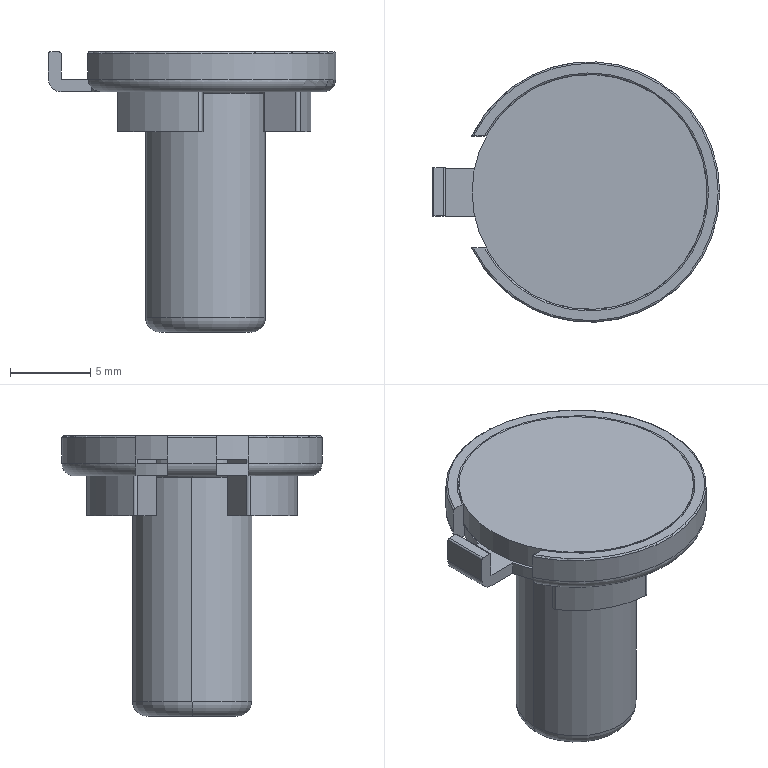NC program | NX | posted with a generic post | part box 17.958 x 16.273 x 17.5 mm
Lines 4508 to 5494 of 9718:
(ZLEVEL_PROFILE_COPY_1_1 , TOOL : D1)
N8984 T12 M6
N8986 G54
N8988 G17 G0 G90 X-4.003 Y4.335 S6500 M3
N8990 G43 Z10. H12
N8992 Z-1.715
N8994 G94 G1 X-4.172 Y4.382 F850.
N8996 X-4.208 Y4.395
N8998 X-4.245 Y4.386
N9000 X-4.269 Y4.357
N9002 G3 X-4.891 Y3.646 R6.1
N9004 G1 X-3.528 Y2.794
N9006 G2 X-3.001 Y3.354 R4.5
N9008 G1 X-2.97 Y3.376
N9010 X-2.958 Y3.413
N9012 X-2.969 Y3.449
N9014 X-3.004 Y3.615
N9016 G0 X-4.003 Y4.335 Z-1.73
N9018 G1 X-4.172 Y4.382
N9020 X-4.208 Y4.395
N9022 X-4.245 Y4.386
N9024 X-4.269 Y4.357
N9026 G3 X-4.891 Y3.646 R6.1
N9028 G1 X-3.528 Y2.794
N9030 G2 X-3.001 Y3.354 R4.5
N9032 G1 X-2.97 Y3.376
N9034 X-2.958 Y3.413
N9036 X-2.969 Y3.449
N9038 X-3.004 Y3.615
N9040 G0 X-4.003 Y4.335 Z-1.744
N9042 G1 X-4.172 Y4.382
N9044 X-4.208 Y4.395
N9046 X-4.245 Y4.386
N9048 X-4.269 Y4.357
N9050 G3 X-4.891 Y3.646 R6.1
N9052 G1 X-3.528 Y2.794
N9054 G2 X-3.001 Y3.354 R4.5
N9056 G1 X-2.97 Y3.376
N9058 X-2.958 Y3.413
N9060 X-2.969 Y3.449
N9062 X-3.004 Y3.615
N9064 G0 X-4.003 Y4.335 Z-1.759
N9066 G1 X-4.172 Y4.382
N9068 X-4.208 Y4.395
N9070 X-4.245 Y4.386
N9072 X-4.269 Y4.357
N9074 G3 X-4.891 Y3.646 R6.1
N9076 G1 X-3.528 Y2.794
N9078 G2 X-3.001 Y3.354 R4.5
N9080 G1 X-2.97 Y3.376
N9082 X-2.958 Y3.413
N9084 X-2.969 Y3.449
N9086 X-3.004 Y3.615
N9088 G0 X-4.003 Y4.335 Z-1.774
N9090 G1 X-4.172 Y4.382
N9092 X-4.208 Y4.395
N9094 X-4.245 Y4.386
N9096 X-4.269 Y4.357
N9098 G3 X-4.891 Y3.646 R6.1
N9100 G1 X-3.528 Y2.794
N9102 G2 X-3.001 Y3.354 R4.5
N9104 G1 X-2.97 Y3.376
N9106 X-2.958 Y3.413
N9108 X-2.969 Y3.449
N9110 X-3.004 Y3.615
N9112 G0 X-4.003 Y4.335 Z-1.789
N9114 G1 X-4.172 Y4.382
N9116 X-4.208 Y4.395
N9118 X-4.245 Y4.386
N9120 X-4.269 Y4.357
N9122 G3 X-4.891 Y3.646 R6.1
N9124 G1 X-3.528 Y2.794
N9126 G2 X-3.001 Y3.354 R4.5
N9128 G1 X-2.97 Y3.376
N9130 X-2.958 Y3.413
N9132 X-2.969 Y3.449
N9134 X-3.004 Y3.615
N9136 G0 X-4.003 Y4.335 Z-1.804
N9138 G1 X-4.172 Y4.382
N9140 X-4.208 Y4.395
N9142 X-4.245 Y4.386
N9144 X-4.269 Y4.357
N9146 G3 X-4.891 Y3.646 R6.1
N9148 G1 X-3.528 Y2.794
N9150 G2 X-3.001 Y3.354 R4.5
N9152 G1 X-2.97 Y3.376
N9154 X-2.958 Y3.413
N9156 X-2.969 Y3.449
N9158 X-3.004 Y3.615
N9160 G0 X-4.003 Y4.335 Z-1.819
N9162 G1 X-4.172 Y4.382
N9164 X-4.208 Y4.395
N9166 X-4.245 Y4.386
N9168 X-4.269 Y4.357
N9170 G3 X-4.891 Y3.646 R6.1
N9172 G1 X-3.528 Y2.794
N9174 G2 X-3.001 Y3.354 R4.5
N9176 G1 X-2.97 Y3.376
N9178 X-2.958 Y3.413
N9180 X-2.969 Y3.449
N9182 X-3.004 Y3.615
N9184 G0 X-4.003 Y4.335 Z-1.833
N9186 G1 X-4.172 Y4.382
N9188 X-4.208 Y4.395
N9190 X-4.245 Y4.386
N9192 X-4.269 Y4.357
N9194 G3 X-4.891 Y3.646 R6.1
N9196 G1 X-3.528 Y2.794
N9198 G2 X-3.001 Y3.354 R4.5
N9200 G1 X-2.97 Y3.376
N9202 X-2.958 Y3.413
N9204 X-2.969 Y3.449
N9206 X-3.004 Y3.615
N9208 G0 X-4.003 Y4.335 Z-1.848
N9210 G1 X-4.172 Y4.382
N9212 X-4.208 Y4.395
N9214 X-4.245 Y4.386
N9216 X-4.269 Y4.357
N9218 G3 X-4.891 Y3.646 R6.1
N9220 G1 X-3.528 Y2.794
N9222 G2 X-3.001 Y3.354 R4.5
N9224 G1 X-2.97 Y3.376
N9226 X-2.958 Y3.413
N9228 X-2.969 Y3.449
N9230 X-3.004 Y3.615
N9232 G0 X-4.003 Y4.335 Z-1.863
N9234 G1 X-4.172 Y4.382
N9236 X-4.208 Y4.395
N9238 X-4.245 Y4.386
N9240 X-4.269 Y4.357
N9242 G3 X-4.891 Y3.646 R6.1
N9244 G1 X-3.528 Y2.794
N9246 G2 X-3.001 Y3.354 R4.5
N9248 G1 X-2.97 Y3.376
N9250 X-2.958 Y3.413
N9252 X-2.969 Y3.449
N9254 X-3.004 Y3.615
N9256 G0 X-4.003 Y4.335 Z-1.878
N9258 G1 X-4.172 Y4.382
N9260 X-4.208 Y4.395
N9262 X-4.245 Y4.386
N9264 X-4.269 Y4.357
N9266 G3 X-4.891 Y3.646 R6.1
N9268 G1 X-3.528 Y2.794
N9270 G2 X-3.001 Y3.354 R4.5
N9272 G1 X-2.97 Y3.376
N9274 X-2.958 Y3.413
N9276 X-2.969 Y3.449
N9278 X-3.004 Y3.615
N9280 G0 X-4.003 Y4.335 Z-1.893
N9282 G1 X-4.172 Y4.382
N9284 X-4.208 Y4.395
N9286 X-4.245 Y4.386
N9288 X-4.269 Y4.357
N9290 G3 X-4.891 Y3.646 R6.1
N9292 G1 X-3.528 Y2.794
N9294 G2 X-3.001 Y3.354 R4.5
N9296 G1 X-2.97 Y3.376
N9298 X-2.958 Y3.413
N9300 X-2.969 Y3.449
N9302 X-3.004 Y3.615
N9304 G0 X-4.003 Y4.335 Z-1.907
N9306 G1 X-4.172 Y4.382
N9308 X-4.208 Y4.395
N9310 X-4.245 Y4.386
N9312 X-4.269 Y4.357
N9314 G3 X-4.891 Y3.646 R6.1
N9316 G1 X-3.528 Y2.794
N9318 G2 X-3.001 Y3.354 R4.5
N9320 G1 X-2.97 Y3.376
N9322 X-2.958 Y3.413
N9324 X-2.969 Y3.449
N9326 X-3.004 Y3.615
N9328 G0 X-4.003 Y4.335 Z-1.922
N9330 G1 X-4.172 Y4.382
N9332 X-4.208 Y4.395
N9334 X-4.245 Y4.386
N9336 X-4.269 Y4.357
N9338 G3 X-4.891 Y3.646 R6.1
N9340 G1 X-3.528 Y2.794
N9342 G2 X-3.001 Y3.354 R4.5
N9344 G1 X-2.97 Y3.376
N9346 X-2.958 Y3.413
N9348 X-2.969 Y3.449
N9350 X-3.004 Y3.615
N9352 G0 X-4.003 Y4.335 Z-1.937
N9354 G1 X-4.172 Y4.382
N9356 X-4.208 Y4.395
N9358 X-4.245 Y4.386
N9360 X-4.269 Y4.357
N9362 G3 X-4.891 Y3.646 R6.1
N9364 G1 X-3.528 Y2.794
N9366 G2 X-3.001 Y3.354 R4.5
N9368 G1 X-2.97 Y3.376
N9370 X-2.958 Y3.413
N9372 X-2.969 Y3.449
N9374 X-3.004 Y3.615
N9376 G0 X-4.003 Y4.335 Z-1.952
N9378 G1 X-4.172 Y4.382
N9380 X-4.208 Y4.395
N9382 X-4.245 Y4.386
N9384 X-4.269 Y4.357
N9386 G3 X-4.891 Y3.646 R6.1
N9388 G1 X-3.528 Y2.794
N9390 G2 X-3.001 Y3.354 R4.5
N9392 G1 X-2.97 Y3.376
N9394 X-2.958 Y3.413
N9396 X-2.969 Y3.449
N9398 X-3.004 Y3.615
N9400 G0 X-4.003 Y4.335 Z-1.967
N9402 G1 X-4.172 Y4.382
N9404 X-4.208 Y4.395
N9406 X-4.245 Y4.386
N9408 X-4.269 Y4.357
N9410 G3 X-4.891 Y3.646 R6.1
N9412 G1 X-3.528 Y2.794
N9414 G2 X-3.001 Y3.354 R4.5
N9416 G1 X-2.97 Y3.376
N9418 X-2.958 Y3.413
N9420 X-2.969 Y3.449
N9422 X-3.004 Y3.615
N9424 G0 X-4.003 Y4.335 Z-1.981
N9426 G1 X-4.172 Y4.382
N9428 X-4.208 Y4.395
N9430 X-4.245 Y4.386
N9432 X-4.269 Y4.357
N9434 G3 X-4.891 Y3.646 R6.1
N9436 G1 X-3.528 Y2.794
N9438 G2 X-3.001 Y3.354 R4.5
N9440 G1 X-2.97 Y3.376
N9442 X-2.958 Y3.413
N9444 X-2.969 Y3.449
N9446 X-3.004 Y3.615
N9448 G0 X-4.003 Y4.335 Z-1.996
N9450 G1 X-4.172 Y4.382
N9452 X-4.208 Y4.395
N9454 X-4.245 Y4.386
N9456 X-4.269 Y4.357
N9458 G3 X-4.891 Y3.646 R6.1
N9460 G1 X-3.528 Y2.794
N9462 G2 X-3.001 Y3.354 R4.5
N9464 G1 X-2.97 Y3.376
N9466 X-2.958 Y3.413
N9468 X-2.969 Y3.449
N9470 X-3.004 Y3.615
N9472 G0 X-4.003 Y4.335 Z-2.011
N9474 G1 X-4.172 Y4.382
N9476 X-4.208 Y4.395
N9478 X-4.245 Y4.386
N9480 X-4.269 Y4.357
N9482 G3 X-4.891 Y3.646 R6.1
N9484 G1 X-3.528 Y2.794
N9486 G2 X-3.001 Y3.354 R4.5
N9488 G1 X-2.97 Y3.376
N9490 X-2.958 Y3.413
N9492 X-2.969 Y3.449
N9494 X-3.004 Y3.615
N9496 G0 X-4.003 Y4.335 Z-2.026
N9498 G1 X-4.172 Y4.382
N9500 X-4.208 Y4.395
N9502 X-4.245 Y4.386
N9504 X-4.269 Y4.357
N9506 G3 X-4.891 Y3.646 R6.1
N9508 G1 X-3.528 Y2.794
N9510 G2 X-3.001 Y3.354 R4.5
N9512 G1 X-2.97 Y3.376
N9514 X-2.958 Y3.413
N9516 X-2.969 Y3.449
N9518 X-3.004 Y3.615
N9520 G0 X-4.003 Y4.335 Z-2.041
N9522 G1 X-4.172 Y4.382
N9524 X-4.208 Y4.395
N9526 X-4.245 Y4.386
N9528 X-4.269 Y4.357
N9530 G3 X-4.891 Y3.646 R6.1
N9532 G1 X-3.528 Y2.794
N9534 G2 X-3.001 Y3.354 R4.5
N9536 G1 X-2.97 Y3.376
N9538 X-2.958 Y3.413
N9540 X-2.969 Y3.449
N9542 X-3.004 Y3.615
N9544 G0 X-4.003 Y4.335 Z-2.056
N9546 G1 X-4.172 Y4.382
N9548 X-4.208 Y4.395
N9550 X-4.245 Y4.386
N9552 X-4.269 Y4.357
N9554 G3 X-4.891 Y3.646 R6.1
N9556 G1 X-3.528 Y2.794
N9558 G2 X-3.001 Y3.354 R4.5
N9560 G1 X-2.97 Y3.376
N9562 X-2.958 Y3.413
N9564 X-2.969 Y3.449
N9566 X-3.004 Y3.615
N9568 G0 X-4.003 Y4.335 Z-2.07
N9570 G1 X-4.172 Y4.382
N9572 X-4.208 Y4.395
N9574 X-4.245 Y4.386
N9576 X-4.269 Y4.357
N9578 G3 X-4.891 Y3.646 R6.1
N9580 G1 X-3.528 Y2.794
N9582 G2 X-3.001 Y3.354 R4.5
N9584 G1 X-2.97 Y3.376
N9586 X-2.958 Y3.413
N9588 X-2.969 Y3.449
N9590 X-3.004 Y3.615
N9592 G0 X-4.003 Y4.335 Z-2.085
N9594 G1 X-4.172 Y4.382
N9596 X-4.208 Y4.395
N9598 X-4.245 Y4.386
N9600 X-4.269 Y4.357
N9602 G3 X-4.891 Y3.646 R6.1
N9604 G1 X-3.528 Y2.794
N9606 G2 X-3.001 Y3.354 R4.5
N9608 G1 X-2.97 Y3.376
N9610 X-2.958 Y3.413
N9612 X-2.969 Y3.449
N9614 X-3.004 Y3.615
N9616 G0 X-4.003 Y4.335 Z-2.1
N9618 G1 X-4.172 Y4.382
N9620 X-4.208 Y4.395
N9622 X-4.245 Y4.386
N9624 X-4.269 Y4.357
N9626 G3 X-4.891 Y3.646 R6.1
N9628 G1 X-3.528 Y2.794
N9630 G2 X-3.001 Y3.354 R4.5
N9632 G1 X-2.97 Y3.376
N9634 X-2.958 Y3.413
N9636 X-2.969 Y3.449
N9638 X-3.004 Y3.615
N9640 G0 X-4.003 Y4.335 Z-2.115
N9642 G1 X-4.172 Y4.382
N9644 X-4.208 Y4.395
N9646 X-4.245 Y4.386
N9648 X-4.269 Y4.357
N9650 G3 X-4.891 Y3.646 R6.1
N9652 G1 X-3.528 Y2.794
N9654 G2 X-3.001 Y3.354 R4.5
N9656 G1 X-2.97 Y3.376
N9658 X-2.958 Y3.413
N9660 X-2.969 Y3.449
N9662 X-3.004 Y3.615
N9664 G0 X-4.003 Y4.335 Z-2.13
N9666 G1 X-4.172 Y4.382
N9668 X-4.208 Y4.395
N9670 X-4.245 Y4.386
N9672 X-4.269 Y4.357
N9674 G3 X-4.891 Y3.646 R6.1
N9676 G1 X-3.528 Y2.794
N9678 G2 X-3.001 Y3.354 R4.5
N9680 G1 X-2.97 Y3.376
N9682 X-2.958 Y3.413
N9684 X-2.969 Y3.449
N9686 X-3.004 Y3.615
N9688 G0 X-4.003 Y4.335 Z-2.144
N9690 G1 X-4.172 Y4.382
N9692 X-4.208 Y4.395
N9694 X-4.245 Y4.386
N9696 X-4.269 Y4.357
N9698 G3 X-4.891 Y3.646 R6.1
N9700 G1 X-3.528 Y2.794
N9702 G2 X-3.001 Y3.354 R4.5
N9704 G1 X-2.97 Y3.376
N9706 X-2.958 Y3.413
N9708 X-2.969 Y3.449
N9710 X-3.004 Y3.615
N9712 G0 X-4.003 Y4.335 Z-2.159
N9714 G1 X-4.172 Y4.382
N9716 X-4.208 Y4.395
N9718 X-4.245 Y4.386
N9720 X-4.269 Y4.357
N9722 G3 X-4.891 Y3.646 R6.1
N9724 G1 X-3.528 Y2.794
N9726 G2 X-3.001 Y3.354 R4.5
N9728 G1 X-2.97 Y3.376
N9730 X-2.958 Y3.413
N9732 X-2.969 Y3.449
N9734 X-3.004 Y3.615
N9736 G0 X-4.003 Y4.335 Z-2.174
N9738 G1 X-4.172 Y4.382
N9740 X-4.208 Y4.395
N9742 X-4.245 Y4.386
N9744 X-4.269 Y4.357
N9746 G3 X-4.891 Y3.646 R6.1
N9748 G1 X-3.528 Y2.794
N9750 G2 X-3.001 Y3.354 R4.5
N9752 G1 X-2.97 Y3.376
N9754 X-2.958 Y3.413
N9756 X-2.969 Y3.449
N9758 X-3.004 Y3.615
N9760 G0 X-4.003 Y4.335 Z-2.189
N9762 G1 X-4.172 Y4.382
N9764 X-4.208 Y4.395
N9766 X-4.245 Y4.386
N9768 X-4.269 Y4.357
N9770 G3 X-4.891 Y3.646 R6.1
N9772 G1 X-3.528 Y2.794
N9774 G2 X-3.001 Y3.354 R4.5
N9776 G1 X-2.97 Y3.376
N9778 X-2.958 Y3.413
N9780 X-2.969 Y3.449
N9782 X-3.004 Y3.615
N9784 G0 X-4.003 Y4.335 Z-2.204
N9786 G1 X-4.172 Y4.382
N9788 X-4.208 Y4.395
N9790 X-4.245 Y4.386
N9792 X-4.269 Y4.357
N9794 G3 X-4.891 Y3.646 R6.1
N9796 G1 X-3.528 Y2.794
N9798 G2 X-3.001 Y3.354 R4.5
N9800 G1 X-2.97 Y3.376
N9802 X-2.958 Y3.413
N9804 X-2.969 Y3.449
N9806 X-3.004 Y3.615
N9808 G0 X-4.003 Y4.335 Z-2.219
N9810 G1 X-4.172 Y4.382
N9812 X-4.208 Y4.395
N9814 X-4.245 Y4.386
N9816 X-4.269 Y4.357
N9818 G3 X-4.891 Y3.646 R6.1
N9820 G1 X-3.528 Y2.794
N9822 G2 X-3.001 Y3.354 R4.5
N9824 G1 X-2.97 Y3.376
N9826 X-2.958 Y3.413
N9828 X-2.969 Y3.449
N9830 X-3.004 Y3.615
N9832 G0 X-4.003 Y4.335 Z-2.233
N9834 G1 X-4.172 Y4.382
N9836 X-4.208 Y4.395
N9838 X-4.245 Y4.386
N9840 X-4.269 Y4.357
N9842 G3 X-4.891 Y3.646 R6.1
N9844 G1 X-3.528 Y2.794
N9846 G2 X-3.001 Y3.354 R4.5
N9848 G1 X-2.97 Y3.376
N9850 X-2.958 Y3.413
N9852 X-2.969 Y3.449
N9854 X-3.004 Y3.615
N9856 G0 X-4.003 Y4.335 Z-2.248
N9858 G1 X-4.172 Y4.382
N9860 X-4.208 Y4.395
N9862 X-4.245 Y4.386
N9864 X-4.269 Y4.357
N9866 G3 X-4.891 Y3.646 R6.1
N9868 G1 X-3.528 Y2.794
N9870 G2 X-3.001 Y3.354 R4.5
N9872 G1 X-2.97 Y3.376
N9874 X-2.958 Y3.413
N9876 X-2.969 Y3.449
N9878 X-3.004 Y3.615
N9880 G0 X-4.003 Y4.335 Z-2.263
N9882 G1 X-4.172 Y4.382
N9884 X-4.208 Y4.395
N9886 X-4.245 Y4.386
N9888 X-4.269 Y4.357
N9890 G3 X-4.891 Y3.646 R6.1
N9892 G1 X-3.528 Y2.794
N9894 G2 X-3.001 Y3.354 R4.5
N9896 G1 X-2.97 Y3.376
N9898 X-2.958 Y3.413
N9900 X-2.969 Y3.449
N9902 X-3.004 Y3.615
N9904 G0 X-4.003 Y4.335 Z-2.278
N9906 G1 X-4.172 Y4.382
N9908 X-4.208 Y4.395
N9910 X-4.245 Y4.386
N9912 X-4.269 Y4.357
N9914 G3 X-4.891 Y3.646 R6.1
N9916 G1 X-3.528 Y2.794
N9918 G2 X-3.001 Y3.354 R4.5
N9920 G1 X-2.97 Y3.376
N9922 X-2.958 Y3.413
N9924 X-2.969 Y3.449
N9926 X-3.004 Y3.615
N9928 G0 X-4.003 Y4.335 Z-2.293
N9930 G1 X-4.172 Y4.382
N9932 X-4.208 Y4.395
N9934 X-4.245 Y4.386
N9936 X-4.269 Y4.357
N9938 G3 X-4.891 Y3.646 R6.1
N9940 G1 X-3.528 Y2.794
N9942 G2 X-3.001 Y3.354 R4.5
N9944 G1 X-2.97 Y3.376
N9946 X-2.958 Y3.413
N9948 X-2.969 Y3.449
N9950 X-3.004 Y3.615
N9952 G0 X-4.003 Y4.335 Z-2.307
N9954 G1 X-4.172 Y4.382
N9956 X-4.208 Y4.395
N9958 X-4.245 Y4.386
N9960 X-4.269 Y4.357
N9962 G3 X-4.891 Y3.646 R6.1
N9964 G1 X-3.528 Y2.794
N9966 G2 X-3.001 Y3.354 R4.5
N9968 G1 X-2.97 Y3.376
N9970 X-2.958 Y3.413
N9972 X-2.969 Y3.449
N9974 X-3.004 Y3.615
N9976 G0 X-4.003 Y4.335 Z-2.322
N9978 G1 X-4.172 Y4.382
N9980 X-4.208 Y4.395
N9982 X-4.245 Y4.386
N9984 X-4.269 Y4.357
N9986 G3 X-4.891 Y3.646 R6.1
N9988 G1 X-3.528 Y2.794
N9990 G2 X-3.001 Y3.354 R4.5
N9992 G1 X-2.97 Y3.376
N9994 X-2.958 Y3.413
N9996 X-2.969 Y3.449
N9998 X-3.004 Y3.615
N10000 G0 X-4.003 Y4.335 Z-2.337
N10002 G1 X-4.172 Y4.382
N10004 X-4.208 Y4.395
N10006 X-4.245 Y4.386
N10008 X-4.269 Y4.357
N10010 G3 X-4.891 Y3.646 R6.1
N10012 G1 X-3.528 Y2.794
N10014 G2 X-3.001 Y3.354 R4.5
N10016 G1 X-2.97 Y3.376
N10018 X-2.958 Y3.413
N10020 X-2.969 Y3.449
N10022 X-3.004 Y3.615
N10024 G0 X-4.003 Y4.335 Z-2.352
N10026 G1 X-4.172 Y4.382
N10028 X-4.208 Y4.395
N10030 X-4.245 Y4.386
N10032 X-4.269 Y4.357
N10034 G3 X-4.891 Y3.646 R6.1
N10036 G1 X-3.528 Y2.794
N10038 G2 X-3.001 Y3.354 R4.5
N10040 G1 X-2.97 Y3.376
N10042 X-2.958 Y3.413
N10044 X-2.969 Y3.449
N10046 X-3.004 Y3.615
N10048 G0 X-4.003 Y4.335 Z-2.367
N10050 G1 X-4.172 Y4.382
N10052 X-4.208 Y4.395
N10054 X-4.245 Y4.386
N10056 X-4.269 Y4.357
N10058 G3 X-4.891 Y3.646 R6.1
N10060 G1 X-3.528 Y2.794
N10062 G2 X-3.001 Y3.354 R4.5
N10064 G1 X-2.97 Y3.376
N10066 X-2.958 Y3.413
N10068 X-2.969 Y3.449
N10070 X-3.004 Y3.615
N10072 G0 X-4.003 Y4.335 Z-2.381
N10074 G1 X-4.172 Y4.382
N10076 X-4.208 Y4.395
N10078 X-4.245 Y4.386
N10080 X-4.269 Y4.357
N10082 G3 X-4.891 Y3.646 R6.1
N10084 G1 X-3.528 Y2.794
N10086 G2 X-3.001 Y3.354 R4.5
N10088 G1 X-2.97 Y3.376
N10090 X-2.958 Y3.413
N10092 X-2.969 Y3.449
N10094 X-3.004 Y3.615
N10096 G0 X-4.003 Y4.335 Z-2.396
N10098 G1 X-4.172 Y4.382
N10100 X-4.208 Y4.395
N10102 X-4.245 Y4.386
N10104 X-4.269 Y4.357
N10106 G3 X-4.891 Y3.646 R6.1
N10108 G1 X-3.528 Y2.794
N10110 G2 X-3.001 Y3.354 R4.5
N10112 G1 X-2.97 Y3.376
N10114 X-2.958 Y3.413
N10116 X-2.969 Y3.449
N10118 X-3.004 Y3.615
N10120 G0 X-4.003 Y4.335 Z-2.411
N10122 G1 X-4.172 Y4.382
N10124 X-4.208 Y4.395
N10126 X-4.245 Y4.386
N10128 X-4.269 Y4.357
N10130 G3 X-4.891 Y3.646 R6.1
N10132 G1 X-3.528 Y2.794
N10134 G2 X-3.001 Y3.354 R4.5
N10136 G1 X-2.97 Y3.376
N10138 X-2.958 Y3.413
N10140 X-2.969 Y3.449
N10142 X-3.004 Y3.615
N10144 G0 X-4.003 Y4.335 Z-2.426
N10146 G1 X-4.172 Y4.382
N10148 X-4.208 Y4.395
N10150 X-4.245 Y4.386
N10152 X-4.269 Y4.357
N10154 G3 X-4.891 Y3.646 R6.1
N10156 G1 X-3.528 Y2.794
N10158 G2 X-3.001 Y3.354 R4.5
N10160 G1 X-2.97 Y3.376
N10162 X-2.958 Y3.413
N10164 X-2.969 Y3.449
N10166 X-3.004 Y3.615
N10168 G0 X-4.003 Y4.335 Z-2.441
N10170 G1 X-4.172 Y4.382
N10172 X-4.208 Y4.395
N10174 X-4.245 Y4.386
N10176 X-4.269 Y4.357
N10178 G3 X-4.891 Y3.646 R6.1
N10180 G1 X-3.528 Y2.794
N10182 G2 X-3.001 Y3.354 R4.5
N10184 G1 X-2.97 Y3.376
N10186 X-2.958 Y3.413
N10188 X-2.969 Y3.449
N10190 X-3.004 Y3.615
N10192 G0 X-4.003 Y4.335 Z-2.456
N10194 G1 X-4.172 Y4.382
N10196 X-4.208 Y4.395
N10198 X-4.245 Y4.386
N10200 X-4.269 Y4.357
N10202 G3 X-4.891 Y3.646 R6.1
N10204 G1 X-3.528 Y2.794
N10206 G2 X-3.001 Y3.354 R4.5
N10208 G1 X-2.97 Y3.376
N10210 X-2.958 Y3.413
N10212 X-2.969 Y3.449
N10214 X-3.004 Y3.615
N10216 G0 X-4.003 Y4.335 Z-2.47
N10218 G1 X-4.172 Y4.382
N10220 X-4.208 Y4.395
N10222 X-4.245 Y4.386
N10224 X-4.269 Y4.357
N10226 G3 X-4.891 Y3.646 R6.1
N10228 G1 X-3.528 Y2.794
N10230 G2 X-3.001 Y3.354 R4.5
N10232 G1 X-2.97 Y3.376
N10234 X-2.958 Y3.413
N10236 X-2.969 Y3.449
N10238 X-3.004 Y3.615
N10240 G0 X-4.003 Y4.335 Z-2.485
N10242 G1 X-4.172 Y4.382
N10244 X-4.208 Y4.395
N10246 X-4.245 Y4.386
N10248 X-4.269 Y4.357
N10250 G3 X-4.891 Y3.646 R6.1
N10252 G1 X-3.528 Y2.794
N10254 G2 X-3.001 Y3.354 R4.5
N10256 G1 X-2.97 Y3.376
N10258 X-2.958 Y3.413
N10260 X-2.969 Y3.449
N10262 X-3.004 Y3.615
N10264 G0 X-4.003 Y4.335 Z-2.5
N10266 G1 X-4.172 Y4.382
N10268 X-4.208 Y4.395
N10270 X-4.245 Y4.386
N10272 X-4.269 Y4.357
N10274 G3 X-4.891 Y3.646 R6.1
N10276 G1 X-3.528 Y2.794
N10278 G2 X-3.001 Y3.354 R4.5
N10280 G1 X-2.97 Y3.376
N10282 X-2.958 Y3.413
N10284 X-2.969 Y3.449
N10286 X-3.004 Y3.615
N10288 G0 Z10.
N10290 X-1.628 Y4.409
N10292 Z-1.715
N10294 G1 X-1.502 Y4.296
N10296 X-1.476 Y4.268
N10298 X-1.439 Y4.26
N10300 X-1.404 Y4.275
N10302 G2 X-0.656 Y4.452 R4.5
N10304 G1 X-0.712 Y6.058
N10306 G3 X-1.639 Y5.876 R6.1
N10308 G1 X-1.676 Y5.869
N10310 X-1.703 Y5.842
N10312 X-1.709 Y5.804
N10314 X-1.753 Y5.634
N10316 G0 X-1.628 Y4.409 Z-1.73
N10318 G1 X-1.502 Y4.296
N10320 X-1.476 Y4.268
N10322 X-1.439 Y4.26
N10324 X-1.404 Y4.275
N10326 G2 X-0.656 Y4.452 R4.5
N10328 G1 X-0.712 Y6.058
N10330 G3 X-1.639 Y5.876 R6.1
N10332 G1 X-1.676 Y5.869
N10334 X-1.703 Y5.842
N10336 X-1.709 Y5.804
N10338 X-1.753 Y5.634
N10340 G0 X-1.628 Y4.409 Z-1.744
N10342 G1 X-1.502 Y4.296
N10344 X-1.476 Y4.268
N10346 X-1.439 Y4.26
N10348 X-1.404 Y4.275
N10350 G2 X-0.656 Y4.452 R4.5
N10352 G1 X-0.712 Y6.058
N10354 G3 X-1.639 Y5.876 R6.1
N10356 G1 X-1.676 Y5.869
N10358 X-1.703 Y5.842
N10360 X-1.709 Y5.804
N10362 X-1.753 Y5.634
N10364 G0 X-1.628 Y4.409 Z-1.759
N10366 G1 X-1.502 Y4.296
N10368 X-1.476 Y4.268
N10370 X-1.439 Y4.26
N10372 X-1.404 Y4.275
N10374 G2 X-0.656 Y4.452 R4.5
N10376 G1 X-0.712 Y6.058
N10378 G3 X-1.639 Y5.876 R6.1
N10380 G1 X-1.676 Y5.869
N10382 X-1.703 Y5.842
N10384 X-1.709 Y5.804
N10386 X-1.753 Y5.634
N10388 G0 X-1.628 Y4.409 Z-1.774
N10390 G1 X-1.502 Y4.296
N10392 X-1.476 Y4.268
N10394 X-1.439 Y4.26
N10396 X-1.404 Y4.275
N10398 G2 X-0.656 Y4.452 R4.5
N10400 G1 X-0.712 Y6.058
N10402 G3 X-1.639 Y5.876 R6.1
N10404 G1 X-1.676 Y5.869
N10406 X-1.703 Y5.842
N10408 X-1.709 Y5.804
N10410 X-1.753 Y5.634
N10412 G0 X-1.628 Y4.409 Z-1.789
N10414 G1 X-1.502 Y4.296
N10416 X-1.476 Y4.268
N10418 X-1.439 Y4.26
N10420 X-1.404 Y4.275
N10422 G2 X-0.656 Y4.452 R4.5
N10424 G1 X-0.712 Y6.058
N10426 G3 X-1.639 Y5.876 R6.1
N10428 G1 X-1.676 Y5.869
N10430 X-1.703 Y5.842
N10432 X-1.709 Y5.804
N10434 X-1.753 Y5.634
N10436 G0 X-1.628 Y4.409 Z-1.804
N10438 G1 X-1.502 Y4.296
N10440 X-1.476 Y4.268
N10442 X-1.439 Y4.26
N10444 X-1.404 Y4.275
N10446 G2 X-0.656 Y4.452 R4.5
N10448 G1 X-0.712 Y6.058
N10450 G3 X-1.639 Y5.876 R6.1
N10452 G1 X-1.676 Y5.869
N10454 X-1.703 Y5.842
N10456 X-1.709 Y5.804
N10458 X-1.753 Y5.634
N10460 G0 X-1.628 Y4.409 Z-1.819
N10462 G1 X-1.502 Y4.296
N10464 X-1.476 Y4.268
N10466 X-1.439 Y4.26
N10468 X-1.404 Y4.275
N10470 G2 X-0.656 Y4.452 R4.5
N10472 G1 X-0.712 Y6.058
N10474 G3 X-1.639 Y5.876 R6.1
N10476 G1 X-1.676 Y5.869
N10478 X-1.703 Y5.842
N10480 X-1.709 Y5.804
N10482 X-1.753 Y5.634
N10484 G0 X-1.628 Y4.409 Z-1.833
N10486 G1 X-1.502 Y4.296
N10488 X-1.476 Y4.268
N10490 X-1.439 Y4.26
N10492 X-1.404 Y4.275
N10494 G2 X-0.656 Y4.452 R4.5
N10496 G1 X-0.712 Y6.058
N10498 G3 X-1.639 Y5.876 R6.1
N10500 G1 X-1.676 Y5.869
N10502 X-1.703 Y5.842
N10504 X-1.709 Y5.804
N10506 X-1.753 Y5.634
N10508 G0 X-1.628 Y4.409 Z-1.848
N10510 G1 X-1.502 Y4.296
N10512 X-1.476 Y4.268
N10514 X-1.439 Y4.26
N10516 X-1.404 Y4.275
N10518 G2 X-0.656 Y4.452 R4.5
N10520 G1 X-0.712 Y6.058
N10522 G3 X-1.639 Y5.876 R6.1
N10524 G1 X-1.676 Y5.869
N10526 X-1.703 Y5.842
N10528 X-1.709 Y5.804
N10530 X-1.753 Y5.634
N10532 G0 X-1.628 Y4.409 Z-1.863
N10534 G1 X-1.502 Y4.296
N10536 X-1.476 Y4.268
N10538 X-1.439 Y4.26
N10540 X-1.404 Y4.275
N10542 G2 X-0.656 Y4.452 R4.5
N10544 G1 X-0.712 Y6.058
N10546 G3 X-1.639 Y5.876 R6.1
N10548 G1 X-1.676 Y5.869
N10550 X-1.703 Y5.842
N10552 X-1.709 Y5.804
N10554 X-1.753 Y5.634
N10556 G0 X-1.628 Y4.409 Z-1.878
N10558 G1 X-1.502 Y4.296
N10560 X-1.476 Y4.268
N10562 X-1.439 Y4.26
N10564 X-1.404 Y4.275
N10566 G2 X-0.656 Y4.452 R4.5
N10568 G1 X-0.712 Y6.058
N10570 G3 X-1.639 Y5.876 R6.1
N10572 G1 X-1.676 Y5.869
N10574 X-1.703 Y5.842
N10576 X-1.709 Y5.804
N10578 X-1.753 Y5.634
N10580 G0 X-1.628 Y4.409 Z-1.893
N10582 G1 X-1.502 Y4.296
N10584 X-1.476 Y4.268
N10586 X-1.439 Y4.26
N10588 X-1.404 Y4.275
N10590 G2 X-0.656 Y4.452 R4.5
N10592 G1 X-0.712 Y6.058
N10594 G3 X-1.639 Y5.876 R6.1
N10596 G1 X-1.676 Y5.869
N10598 X-1.703 Y5.842
N10600 X-1.709 Y5.804
N10602 X-1.753 Y5.634
N10604 G0 X-1.628 Y4.409 Z-1.907
N10606 G1 X-1.502 Y4.296
N10608 X-1.476 Y4.268
N10610 X-1.439 Y4.26
N10612 X-1.404 Y4.275
N10614 G2 X-0.656 Y4.452 R4.5
N10616 G1 X-0.712 Y6.058
N10618 G3 X-1.639 Y5.876 R6.1
N10620 G1 X-1.676 Y5.869
N10622 X-1.703 Y5.842
N10624 X-1.709 Y5.804
N10626 X-1.753 Y5.634
N10628 G0 X-1.628 Y4.409 Z-1.922
N10630 G1 X-1.502 Y4.296
N10632 X-1.476 Y4.268
N10634 X-1.439 Y4.26
N10636 X-1.404 Y4.275
N10638 G2 X-0.656 Y4.452 R4.5
N10640 G1 X-0.712 Y6.058
N10642 G3 X-1.639 Y5.876 R6.1
N10644 G1 X-1.676 Y5.869
N10646 X-1.703 Y5.842
N10648 X-1.709 Y5.804
N10650 X-1.753 Y5.634
N10652 G0 X-1.628 Y4.409 Z-1.937
N10654 G1 X-1.502 Y4.296
N10656 X-1.476 Y4.268
N10658 X-1.439 Y4.26
N10660 X-1.404 Y4.275
N10662 G2 X-0.656 Y4.452 R4.5
N10664 G1 X-0.712 Y6.058
N10666 G3 X-1.639 Y5.876 R6.1
N10668 G1 X-1.676 Y5.869
N10670 X-1.703 Y5.842
N10672 X-1.709 Y5.804
N10674 X-1.753 Y5.634
N10676 G0 X-1.628 Y4.409 Z-1.952
N10678 G1 X-1.502 Y4.296
N10680 X-1.476 Y4.268
N10682 X-1.439 Y4.26
N10684 X-1.404 Y4.275
N10686 G2 X-0.656 Y4.452 R4.5
N10688 G1 X-0.712 Y6.058
N10690 G3 X-1.639 Y5.876 R6.1
N10692 G1 X-1.676 Y5.869
N10694 X-1.703 Y5.842
N10696 X-1.709 Y5.804
N10698 X-1.753 Y5.634
N10700 G0 X-1.628 Y4.409 Z-1.967
N10702 G1 X-1.502 Y4.296
N10704 X-1.476 Y4.268
N10706 X-1.439 Y4.26
N10708 X-1.404 Y4.275
N10710 G2 X-0.656 Y4.452 R4.5
N10712 G1 X-0.712 Y6.058
N10714 G3 X-1.639 Y5.876 R6.1
N10716 G1 X-1.676 Y5.869
N10718 X-1.703 Y5.842
N10720 X-1.709 Y5.804
N10722 X-1.753 Y5.634
N10724 G0 X-1.628 Y4.409 Z-1.981
N10726 G1 X-1.502 Y4.296
N10728 X-1.476 Y4.268
N10730 X-1.439 Y4.26
N10732 X-1.404 Y4.275
N10734 G2 X-0.656 Y4.452 R4.5
N10736 G1 X-0.712 Y6.058
N10738 G3 X-1.639 Y5.876 R6.1
N10740 G1 X-1.676 Y5.869
N10742 X-1.703 Y5.842
N10744 X-1.709 Y5.804
N10746 X-1.753 Y5.634
N10748 G0 X-1.628 Y4.409 Z-1.996
N10750 G1 X-1.502 Y4.296
N10752 X-1.476 Y4.268
N10754 X-1.439 Y4.26
N10756 X-1.404 Y4.275
N10758 G2 X-0.656 Y4.452 R4.5
N10760 G1 X-0.712 Y6.058
N10762 G3 X-1.639 Y5.876 R6.1
N10764 G1 X-1.676 Y5.869
N10766 X-1.703 Y5.842
N10768 X-1.709 Y5.804
N10770 X-1.753 Y5.634
N10772 G0 X-1.628 Y4.409 Z-2.011
N10774 G1 X-1.502 Y4.296
N10776 X-1.476 Y4.268
N10778 X-1.439 Y4.26
N10780 X-1.404 Y4.275
N10782 G2 X-0.656 Y4.452 R4.5
N10784 G1 X-0.712 Y6.058
N10786 G3 X-1.639 Y5.876 R6.1
N10788 G1 X-1.676 Y5.869
N10790 X-1.703 Y5.842
N10792 X-1.709 Y5.804
N10794 X-1.753 Y5.634
N10796 G0 X-1.628 Y4.409 Z-2.026
N10798 G1 X-1.502 Y4.296
N10800 X-1.476 Y4.268
N10802 X-1.439 Y4.26
N10804 X-1.404 Y4.275
N10806 G2 X-0.656 Y4.452 R4.5
N10808 G1 X-0.712 Y6.058
N10810 G3 X-1.639 Y5.876 R6.1
N10812 G1 X-1.676 Y5.869
N10814 X-1.703 Y5.842
N10816 X-1.709 Y5.804
N10818 X-1.753 Y5.634
N10820 G0 X-1.628 Y4.409 Z-2.041
N10822 G1 X-1.502 Y4.296
N10824 X-1.476 Y4.268
N10826 X-1.439 Y4.26
N10828 X-1.404 Y4.275
N10830 G2 X-0.656 Y4.452 R4.5
N10832 G1 X-0.712 Y6.058
N10834 G3 X-1.639 Y5.876 R6.1
N10836 G1 X-1.676 Y5.869
N10838 X-1.703 Y5.842
N10840 X-1.709 Y5.804
N10842 X-1.753 Y5.634
N10844 G0 X-1.628 Y4.409 Z-2.056
N10846 G1 X-1.502 Y4.296
N10848 X-1.476 Y4.268
N10850 X-1.439 Y4.26
N10852 X-1.404 Y4.275
N10854 G2 X-0.656 Y4.452 R4.5
N10856 G1 X-0.712 Y6.058
N10858 G3 X-1.639 Y5.876 R6.1
N10860 G1 X-1.676 Y5.869
N10862 X-1.703 Y5.842
N10864 X-1.709 Y5.804
N10866 X-1.753 Y5.634
N10868 G0 X-1.628 Y4.409 Z-2.07
N10870 G1 X-1.502 Y4.296
N10872 X-1.476 Y4.268
N10874 X-1.439 Y4.26
N10876 X-1.404 Y4.275
N10878 G2 X-0.656 Y4.452 R4.5
N10880 G1 X-0.712 Y6.058
N10882 G3 X-1.639 Y5.876 R6.1
N10884 G1 X-1.676 Y5.869
N10886 X-1.703 Y5.842
N10888 X-1.709 Y5.804
N10890 X-1.753 Y5.634
N10892 G0 X-1.628 Y4.409 Z-2.085
N10894 G1 X-1.502 Y4.296
N10896 X-1.476 Y4.268
N10898 X-1.439 Y4.26
N10900 X-1.404 Y4.275
N10902 G2 X-0.656 Y4.452 R4.5
N10904 G1 X-0.712 Y6.058
N10906 G3 X-1.639 Y5.876 R6.1
N10908 G1 X-1.676 Y5.869
N10910 X-1.703 Y5.842
N10912 X-1.709 Y5.804
N10914 X-1.753 Y5.634
N10916 G0 X-1.628 Y4.409 Z-2.1
N10918 G1 X-1.502 Y4.296
N10920 X-1.476 Y4.268
N10922 X-1.439 Y4.26
N10924 X-1.404 Y4.275
N10926 G2 X-0.656 Y4.452 R4.5
N10928 G1 X-0.712 Y6.058
N10930 G3 X-1.639 Y5.876 R6.1
N10932 G1 X-1.676 Y5.869
N10934 X-1.703 Y5.842
N10936 X-1.709 Y5.804
N10938 X-1.753 Y5.634
N10940 G0 X-1.628 Y4.409 Z-2.115
N10942 G1 X-1.502 Y4.296
N10944 X-1.476 Y4.268
N10946 X-1.439 Y4.26
N10948 X-1.404 Y4.275
N10950 G2 X-0.656 Y4.452 R4.5